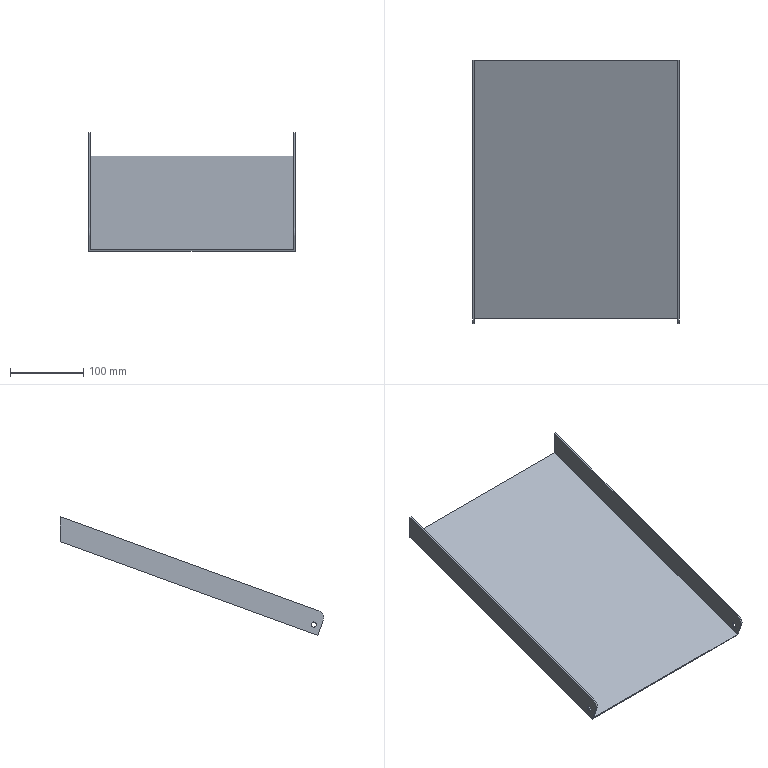Part | NX | features HB 2 | 1 solid | 14 faces | box 281 x 359.033 x 161.773 mm | volume 255383 mm3 | plane 10 | cylinder 4 | commonest cylinder face diameters 7 x2 20 x2
STEP:
#1=CARTESIAN_POINT('',(285.,-685.612,-380.836));
#2=VERTEX_POINT('',#1);
#3=CARTESIAN_POINT('',(285.,-685.612,-377.336));
#4=DIRECTION('',(-1.,0.,0.));
#5=DIRECTION('',(0.,0.,-1.));
#6=AXIS2_PLACEMENT_3D('',#3,#4,#5);
#7=CIRCLE('',#6,3.5);
#8=EDGE_CURVE('',#2,#2,#7,.T.);
#9=ORIENTED_EDGE('',*,*,#8,.T.);
#10=EDGE_LOOP('',(#9));
#11=FACE_BOUND('',#10,.T.);
#12=CARTESIAN_POINT('',(285.,-691.589,-390.154));
#13=VERTEX_POINT('',#12);
#14=CARTESIAN_POINT('',(285.,-340.,-262.186));
#15=VERTEX_POINT('',#14);
#16=CARTESIAN_POINT('',(285.,-379.611,-276.603));
#17=DIRECTION('',(0.,0.9397,0.342));
#18=VECTOR('',#17,1000.);
#19=LINE('',#16,#18);
#20=EDGE_CURVE('',#13,#15,#19,.T.);
#21=ORIENTED_EDGE('',*,*,#20,.T.);
#22=CARTESIAN_POINT('',(285.,-340.,-230.26));
#23=VERTEX_POINT('',#22);
#24=CARTESIAN_POINT('',(285.,-340.,-276.603));
#25=DIRECTION('',(0.,0.,1.));
#26=VECTOR('',#25,1000.);
#27=LINE('',#24,#26);
#28=EDGE_CURVE('',#15,#23,#27,.T.);
#29=ORIENTED_EDGE('',*,*,#28,.T.);
#30=CARTESIAN_POINT('',(285.,-692.453,-358.543));
#31=VERTEX_POINT('',#30);
#32=CARTESIAN_POINT('',(285.,-389.872,-248.412));
#33=DIRECTION('',(0.,-0.9397,-0.342));
#34=VECTOR('',#33,1000.);
#35=LINE('',#32,#34);
#36=EDGE_CURVE('',#23,#31,#35,.T.);
#37=ORIENTED_EDGE('',*,*,#36,.T.);
#38=CARTESIAN_POINT('',(285.,-698.43,-371.36));
#39=VERTEX_POINT('',#38);
#40=CARTESIAN_POINT('',(285.,-689.033,-367.939));
#41=DIRECTION('',(1.,0.,0.));
#42=DIRECTION('',(0.,0.,-1.));
#43=AXIS2_PLACEMENT_3D('',#40,#41,#42);
#44=CIRCLE('',#43,10.);
#45=EDGE_CURVE('',#31,#39,#44,.T.);
#46=ORIENTED_EDGE('',*,*,#45,.T.);
#47=CARTESIAN_POINT('',(285.,-691.589,-390.154));
#48=DIRECTION('',(0.,0.342,-0.9397));
#49=VECTOR('',#48,1000.);
#50=LINE('',#47,#49);
#51=EDGE_CURVE('',#39,#13,#50,.T.);
#52=ORIENTED_EDGE('',*,*,#51,.T.);
#53=EDGE_LOOP('',(#21,#29,#37,#46,#52));
#54=FACE_BOUND('',#53,.T.);
#55=CARTESIAN_POINT('',(285.,-379.611,-276.603));
#56=DIRECTION('',(1.,0.,0.));
#57=DIRECTION('',(0.,0.08716,0.9962));
#58=AXIS2_PLACEMENT_3D('',#55,#56,#57);
#59=PLANE('',#58);
#60=ADVANCED_FACE('',(#11,#54),#59,.T.);
#61=CARTESIAN_POINT('',(562.,-340.,-230.26));
#62=VERTEX_POINT('',#61);
#63=CARTESIAN_POINT('',(564.,-340.,-230.26));
#64=VERTEX_POINT('',#63);
#65=CARTESIAN_POINT('',(562.,-340.,-230.26));
#66=DIRECTION('',(1.,0.,0.));
#67=VECTOR('',#66,1000.);
#68=LINE('',#65,#67);
#69=EDGE_CURVE('',#62,#64,#68,.T.);
#70=ORIENTED_EDGE('',*,*,#69,.F.);
#71=CARTESIAN_POINT('',(562.,-692.453,-358.543));
#72=VERTEX_POINT('',#71);
#73=CARTESIAN_POINT('',(562.,-389.872,-248.412));
#74=DIRECTION('',(0.,-0.9397,-0.342));
#75=VECTOR('',#74,1000.);
#76=LINE('',#73,#75);
#77=EDGE_CURVE('',#62,#72,#76,.T.);
#78=ORIENTED_EDGE('',*,*,#77,.T.);
#79=CARTESIAN_POINT('',(564.,-692.453,-358.543));
#80=VERTEX_POINT('',#79);
#81=CARTESIAN_POINT('',(562.,-692.453,-358.543));
#82=DIRECTION('',(1.,0.,0.));
#83=VECTOR('',#82,1000.);
#84=LINE('',#81,#83);
#85=EDGE_CURVE('',#72,#80,#84,.T.);
#86=ORIENTED_EDGE('',*,*,#85,.T.);
#87=CARTESIAN_POINT('',(564.,-389.872,-248.412));
#88=DIRECTION('',(0.,-0.9397,-0.342));
#89=VECTOR('',#88,1000.);
#90=LINE('',#87,#89);
#91=EDGE_CURVE('',#64,#80,#90,.T.);
#92=ORIENTED_EDGE('',*,*,#91,.F.);
#93=EDGE_LOOP('',(#70,#78,#86,#92));
#94=FACE_BOUND('',#93,.T.);
#95=CARTESIAN_POINT('',(562.,-389.872,-248.412));
#96=DIRECTION('',(0.,0.342,-0.9397));
#97=DIRECTION('',(0.,-0.9397,-0.342));
#98=AXIS2_PLACEMENT_3D('',#95,#96,#97);
#99=PLANE('',#98);
#100=ADVANCED_FACE('',(#94),#99,.F.);
#101=CARTESIAN_POINT('',(562.,-685.307,-373.85));
#102=VERTEX_POINT('',#101);
#103=CARTESIAN_POINT('',(562.,-685.612,-377.336));
#104=DIRECTION('',(1.,0.,0.));
#105=DIRECTION('',(0.,0.08716,0.9962));
#106=AXIS2_PLACEMENT_3D('',#103,#104,#105);
#107=CIRCLE('',#106,3.5);
#108=EDGE_CURVE('',#102,#102,#107,.T.);
#109=ORIENTED_EDGE('',*,*,#108,.T.);
#110=EDGE_LOOP('',(#109));
#111=FACE_BOUND('',#110,.T.);
#112=ORIENTED_EDGE('',*,*,#77,.F.);
#113=CARTESIAN_POINT('',(562.,-340.,-262.186));
#114=VERTEX_POINT('',#113);
#115=CARTESIAN_POINT('',(562.,-340.,-276.603));
#116=DIRECTION('',(0.,0.,-1.));
#117=VECTOR('',#116,1000.);
#118=LINE('',#115,#117);
#119=EDGE_CURVE('',#62,#114,#118,.T.);
#120=ORIENTED_EDGE('',*,*,#119,.T.);
#121=CARTESIAN_POINT('',(562.,-691.589,-390.154));
#122=VERTEX_POINT('',#121);
#123=CARTESIAN_POINT('',(562.,-379.611,-276.603));
#124=DIRECTION('',(0.,-0.9397,-0.342));
#125=VECTOR('',#124,1000.);
#126=LINE('',#123,#125);
#127=EDGE_CURVE('',#114,#122,#126,.T.);
#128=ORIENTED_EDGE('',*,*,#127,.T.);
#129=CARTESIAN_POINT('',(562.,-698.43,-371.36));
#130=VERTEX_POINT('',#129);
#131=CARTESIAN_POINT('',(562.,-691.589,-390.154));
#132=DIRECTION('',(0.,0.342,-0.9397));
#133=VECTOR('',#132,1000.);
#134=LINE('',#131,#133);
#135=EDGE_CURVE('',#130,#122,#134,.T.);
#136=ORIENTED_EDGE('',*,*,#135,.F.);
#137=CARTESIAN_POINT('',(562.,-689.033,-367.939));
#138=DIRECTION('',(-1.,0.,0.));
#139=DIRECTION('',(0.,0.08716,0.9962));
#140=AXIS2_PLACEMENT_3D('',#137,#138,#139);
#141=CIRCLE('',#140,10.);
#142=EDGE_CURVE('',#130,#72,#141,.T.);
#143=ORIENTED_EDGE('',*,*,#142,.T.);
#144=EDGE_LOOP('',(#112,#120,#128,#136,#143));
#145=FACE_BOUND('',#144,.T.);
#146=CARTESIAN_POINT('',(562.,-379.611,-276.603));
#147=DIRECTION('',(-1.,0.,0.));
#148=DIRECTION('',(0.,0.08716,0.9962));
#149=AXIS2_PLACEMENT_3D('',#146,#147,#148);
#150=PLANE('',#149);
#151=ADVANCED_FACE('',(#111,#145),#150,.T.);
#152=CARTESIAN_POINT('',(564.,-685.307,-373.85));
#153=VERTEX_POINT('',#152);
#154=CARTESIAN_POINT('',(564.,-685.612,-377.336));
#155=DIRECTION('',(1.,0.,0.));
#156=DIRECTION('',(0.,0.08716,0.9962));
#157=AXIS2_PLACEMENT_3D('',#154,#155,#156);
#158=CIRCLE('',#157,3.5);
#159=EDGE_CURVE('',#153,#153,#158,.T.);
#160=ORIENTED_EDGE('',*,*,#159,.F.);
#161=EDGE_LOOP('',(#160));
#162=FACE_BOUND('',#161,.T.);
#163=CARTESIAN_POINT('',(564.,-340.,-264.314));
#164=VERTEX_POINT('',#163);
#165=CARTESIAN_POINT('',(564.,-340.,-276.603));
#166=DIRECTION('',(0.,0.,-1.));
#167=VECTOR('',#166,1000.);
#168=LINE('',#165,#167);
#169=EDGE_CURVE('',#64,#164,#168,.T.);
#170=ORIENTED_EDGE('',*,*,#169,.F.);
#171=ORIENTED_EDGE('',*,*,#91,.T.);
#172=CARTESIAN_POINT('',(564.,-698.43,-371.36));
#173=VERTEX_POINT('',#172);
#174=CARTESIAN_POINT('',(564.,-689.033,-367.939));
#175=DIRECTION('',(1.,0.,0.));
#176=DIRECTION('',(0.,0.08716,0.9962));
#177=AXIS2_PLACEMENT_3D('',#174,#175,#176);
#178=CIRCLE('',#177,10.);
#179=EDGE_CURVE('',#80,#173,#178,.T.);
#180=ORIENTED_EDGE('',*,*,#179,.T.);
#181=CARTESIAN_POINT('',(564.,-690.905,-392.033));
#182=VERTEX_POINT('',#181);
#183=CARTESIAN_POINT('',(564.,-691.589,-390.154));
#184=DIRECTION('',(0.,0.342,-0.9397));
#185=VECTOR('',#184,1000.);
#186=LINE('',#183,#185);
#187=EDGE_CURVE('',#173,#182,#186,.T.);
#188=ORIENTED_EDGE('',*,*,#187,.T.);
#189=CARTESIAN_POINT('',(564.,-378.927,-278.482));
#190=DIRECTION('',(0.,0.9397,0.342));
#191=VECTOR('',#190,1000.);
#192=LINE('',#189,#191);
#193=EDGE_CURVE('',#182,#164,#192,.T.);
#194=ORIENTED_EDGE('',*,*,#193,.T.);
#195=EDGE_LOOP('',(#170,#171,#180,#188,#194));
#196=FACE_BOUND('',#195,.T.);
#197=CARTESIAN_POINT('',(564.,-379.611,-276.603));
#198=DIRECTION('',(-1.,0.,0.));
#199=DIRECTION('',(0.,-0.08716,-0.9962));
#200=AXIS2_PLACEMENT_3D('',#197,#198,#199);
#201=PLANE('',#200);
#202=ADVANCED_FACE('',(#162,#196),#201,.F.);
#203=CARTESIAN_POINT('',(283.,-340.,-264.314));
#204=VERTEX_POINT('',#203);
#205=CARTESIAN_POINT('',(283.,-690.905,-392.033));
#206=VERTEX_POINT('',#205);
#207=CARTESIAN_POINT('',(283.,-378.927,-278.482));
#208=DIRECTION('',(0.,-0.9397,-0.342));
#209=VECTOR('',#208,1000.);
#210=LINE('',#207,#209);
#211=EDGE_CURVE('',#204,#206,#210,.T.);
#212=ORIENTED_EDGE('',*,*,#211,.F.);
#213=CARTESIAN_POINT('',(522.,-340.,-264.314));
#214=DIRECTION('',(-1.,0.,0.));
#215=VECTOR('',#214,1000.);
#216=LINE('',#213,#215);
#217=EDGE_CURVE('',#164,#204,#216,.T.);
#218=ORIENTED_EDGE('',*,*,#217,.F.);
#219=ORIENTED_EDGE('',*,*,#193,.F.);
#220=CARTESIAN_POINT('',(522.,-690.905,-392.033));
#221=DIRECTION('',(1.,0.,0.));
#222=VECTOR('',#221,1000.);
#223=LINE('',#220,#222);
#224=EDGE_CURVE('',#206,#182,#223,.T.);
#225=ORIENTED_EDGE('',*,*,#224,.F.);
#226=EDGE_LOOP('',(#212,#218,#219,#225));
#227=FACE_BOUND('',#226,.T.);
#228=CARTESIAN_POINT('',(522.,-378.927,-278.482));
#229=DIRECTION('',(0.,-0.342,0.9397));
#230=DIRECTION('',(-1.,0.,0.));
#231=AXIS2_PLACEMENT_3D('',#228,#229,#230);
#232=PLANE('',#231);
#233=ADVANCED_FACE('',(#227),#232,.F.);
#234=CARTESIAN_POINT('',(522.,-340.,-262.186));
#235=DIRECTION('',(-1.,0.,0.));
#236=VECTOR('',#235,1000.);
#237=LINE('',#234,#236);
#238=EDGE_CURVE('',#114,#15,#237,.T.);
#239=ORIENTED_EDGE('',*,*,#238,.T.);
#240=ORIENTED_EDGE('',*,*,#20,.F.);
#241=CARTESIAN_POINT('',(522.,-691.589,-390.154));
#242=DIRECTION('',(1.,0.,0.));
#243=VECTOR('',#242,1000.);
#244=LINE('',#241,#243);
#245=EDGE_CURVE('',#13,#122,#244,.T.);
#246=ORIENTED_EDGE('',*,*,#245,.T.);
#247=ORIENTED_EDGE('',*,*,#127,.F.);
#248=EDGE_LOOP('',(#239,#240,#246,#247));
#249=FACE_BOUND('',#248,.T.);
#250=CARTESIAN_POINT('',(522.,-379.611,-276.603));
#251=DIRECTION('',(0.,-0.342,0.9397));
#252=DIRECTION('',(-1.,0.,0.));
#253=AXIS2_PLACEMENT_3D('',#250,#251,#252);
#254=PLANE('',#253);
#255=ADVANCED_FACE('',(#249),#254,.T.);
#256=CARTESIAN_POINT('',(283.,-340.,-230.26));
#257=VERTEX_POINT('',#256);
#258=CARTESIAN_POINT('',(275.,-340.,-230.26));
#259=DIRECTION('',(1.,0.,0.));
#260=VECTOR('',#259,1000.);
#261=LINE('',#258,#260);
#262=EDGE_CURVE('',#257,#23,#261,.T.);
#263=ORIENTED_EDGE('',*,*,#262,.F.);
#264=CARTESIAN_POINT('',(283.,-692.453,-358.543));
#265=VERTEX_POINT('',#264);
#266=CARTESIAN_POINT('',(283.,-389.872,-248.412));
#267=DIRECTION('',(0.,-0.9397,-0.342));
#268=VECTOR('',#267,1000.);
#269=LINE('',#266,#268);
#270=EDGE_CURVE('',#257,#265,#269,.T.);
#271=ORIENTED_EDGE('',*,*,#270,.T.);
#272=CARTESIAN_POINT('',(330.,-692.453,-358.543));
#273=DIRECTION('',(1.,0.,0.));
#274=VECTOR('',#273,1000.);
#275=LINE('',#272,#274);
#276=EDGE_CURVE('',#265,#31,#275,.T.);
#277=ORIENTED_EDGE('',*,*,#276,.T.);
#278=ORIENTED_EDGE('',*,*,#36,.F.);
#279=EDGE_LOOP('',(#263,#271,#277,#278));
#280=FACE_BOUND('',#279,.T.);
#281=CARTESIAN_POINT('',(275.,-389.872,-248.412));
#282=DIRECTION('',(0.,0.342,-0.9397));
#283=DIRECTION('',(0.,-0.9397,-0.342));
#284=AXIS2_PLACEMENT_3D('',#281,#282,#283);
#285=PLANE('',#284);
#286=ADVANCED_FACE('',(#280),#285,.F.);
#287=CARTESIAN_POINT('',(283.,-685.612,-380.836));
#288=VERTEX_POINT('',#287);
#289=CARTESIAN_POINT('',(283.,-685.612,-377.336));
#290=DIRECTION('',(1.,0.,0.));
#291=DIRECTION('',(0.,0.,-1.));
#292=AXIS2_PLACEMENT_3D('',#289,#290,#291);
#293=CIRCLE('',#292,3.5);
#294=EDGE_CURVE('',#288,#288,#293,.T.);
#295=ORIENTED_EDGE('',*,*,#294,.T.);
#296=EDGE_LOOP('',(#295));
#297=FACE_BOUND('',#296,.T.);
#298=CARTESIAN_POINT('',(283.,-340.,-276.603));
#299=DIRECTION('',(0.,0.,1.));
#300=VECTOR('',#299,1000.);
#301=LINE('',#298,#300);
#302=EDGE_CURVE('',#204,#257,#301,.T.);
#303=ORIENTED_EDGE('',*,*,#302,.F.);
#304=ORIENTED_EDGE('',*,*,#211,.T.);
#305=CARTESIAN_POINT('',(283.,-698.43,-371.36));
#306=VERTEX_POINT('',#305);
#307=CARTESIAN_POINT('',(283.,-691.589,-390.154));
#308=DIRECTION('',(0.,0.342,-0.9397));
#309=VECTOR('',#308,1000.);
#310=LINE('',#307,#309);
#311=EDGE_CURVE('',#306,#206,#310,.T.);
#312=ORIENTED_EDGE('',*,*,#311,.F.);
#313=CARTESIAN_POINT('',(283.,-689.033,-367.939));
#314=DIRECTION('',(-1.,0.,0.));
#315=DIRECTION('',(0.,0.,-1.));
#316=AXIS2_PLACEMENT_3D('',#313,#314,#315);
#317=CIRCLE('',#316,10.);
#318=EDGE_CURVE('',#306,#265,#317,.T.);
#319=ORIENTED_EDGE('',*,*,#318,.T.);
#320=ORIENTED_EDGE('',*,*,#270,.F.);
#321=EDGE_LOOP('',(#303,#304,#312,#319,#320));
#322=FACE_BOUND('',#321,.T.);
#323=CARTESIAN_POINT('',(283.,-379.611,-276.603));
#324=DIRECTION('',(1.,0.,0.));
#325=DIRECTION('',(0.,0.08716,0.9962));
#326=AXIS2_PLACEMENT_3D('',#323,#324,#325);
#327=PLANE('',#326);
#328=ADVANCED_FACE('',(#297,#322),#327,.F.);
#329=ORIENTED_EDGE('',*,*,#108,.F.);
#330=EDGE_LOOP('',(#329));
#331=FACE_BOUND('',#330,.T.);
#332=ORIENTED_EDGE('',*,*,#159,.T.);
#333=EDGE_LOOP('',(#332));
#334=FACE_BOUND('',#333,.T.);
#335=CARTESIAN_POINT('',(1166.,-685.612,-377.336));
#336=DIRECTION('',(-1.,0.,0.));
#337=DIRECTION('',(0.,-0.08716,-0.9962));
#338=AXIS2_PLACEMENT_3D('',#335,#336,#337);
#339=CYLINDRICAL_SURFACE('',#338,3.5);
#340=ADVANCED_FACE('',(#331,#334),#339,.F.);
#341=ORIENTED_EDGE('',*,*,#142,.F.);
#342=CARTESIAN_POINT('',(522.,-698.43,-371.36));
#343=DIRECTION('',(-1.,0.,0.));
#344=VECTOR('',#343,1000.);
#345=LINE('',#342,#344);
#346=EDGE_CURVE('',#173,#130,#345,.T.);
#347=ORIENTED_EDGE('',*,*,#346,.F.);
#348=ORIENTED_EDGE('',*,*,#179,.F.);
#349=ORIENTED_EDGE('',*,*,#85,.F.);
#350=EDGE_LOOP('',(#341,#347,#348,#349));
#351=FACE_BOUND('',#350,.T.);
#352=CARTESIAN_POINT('',(562.,-689.033,-367.939));
#353=DIRECTION('',(1.,0.,0.));
#354=DIRECTION('',(0.,0.08716,0.9962));
#355=AXIS2_PLACEMENT_3D('',#352,#353,#354);
#356=CYLINDRICAL_SURFACE('',#355,10.);
#357=ADVANCED_FACE('',(#351),#356,.T.);
#358=ORIENTED_EDGE('',*,*,#245,.F.);
#359=ORIENTED_EDGE('',*,*,#51,.F.);
#360=CARTESIAN_POINT('',(588.,-698.43,-371.36));
#361=DIRECTION('',(-1.,0.,0.));
#362=VECTOR('',#361,1000.);
#363=LINE('',#360,#362);
#364=EDGE_CURVE('',#39,#306,#363,.T.);
#365=ORIENTED_EDGE('',*,*,#364,.T.);
#366=ORIENTED_EDGE('',*,*,#311,.T.);
#367=ORIENTED_EDGE('',*,*,#224,.T.);
#368=ORIENTED_EDGE('',*,*,#187,.F.);
#369=ORIENTED_EDGE('',*,*,#346,.T.);
#370=ORIENTED_EDGE('',*,*,#135,.T.);
#371=EDGE_LOOP('',(#358,#359,#365,#366,#367,#368,#369,#370));
#372=FACE_BOUND('',#371,.T.);
#373=CARTESIAN_POINT('',(522.,-691.589,-390.154));
#374=DIRECTION('',(0.,0.9397,0.342));
#375=DIRECTION('',(0.,0.342,-0.9397));
#376=AXIS2_PLACEMENT_3D('',#373,#374,#375);
#377=PLANE('',#376);
#378=ADVANCED_FACE('',(#372),#377,.F.);
#379=ORIENTED_EDGE('',*,*,#45,.F.);
#380=ORIENTED_EDGE('',*,*,#276,.F.);
#381=ORIENTED_EDGE('',*,*,#318,.F.);
#382=ORIENTED_EDGE('',*,*,#364,.F.);
#383=EDGE_LOOP('',(#379,#380,#381,#382));
#384=FACE_BOUND('',#383,.T.);
#385=CARTESIAN_POINT('',(588.,-689.033,-367.939));
#386=DIRECTION('',(-1.,0.,0.));
#387=DIRECTION('',(0.,-0.08716,-0.9962));
#388=AXIS2_PLACEMENT_3D('',#385,#386,#387);
#389=CYLINDRICAL_SURFACE('',#388,10.);
#390=ADVANCED_FACE('',(#384),#389,.T.);
#391=ORIENTED_EDGE('',*,*,#8,.F.);
#392=EDGE_LOOP('',(#391));
#393=FACE_BOUND('',#392,.T.);
#394=ORIENTED_EDGE('',*,*,#294,.F.);
#395=EDGE_LOOP('',(#394));
#396=FACE_BOUND('',#395,.T.);
#397=CARTESIAN_POINT('',(1180.,-685.612,-377.336));
#398=DIRECTION('',(-1.,0.,0.));
#399=DIRECTION('',(0.,-0.08716,-0.9962));
#400=AXIS2_PLACEMENT_3D('',#397,#398,#399);
#401=CYLINDRICAL_SURFACE('',#400,3.5);
#402=ADVANCED_FACE('',(#393,#396),#401,.F.);
#403=ORIENTED_EDGE('',*,*,#69,.T.);
#404=ORIENTED_EDGE('',*,*,#169,.T.);
#405=ORIENTED_EDGE('',*,*,#217,.T.);
#406=ORIENTED_EDGE('',*,*,#302,.T.);
#407=ORIENTED_EDGE('',*,*,#262,.T.);
#408=ORIENTED_EDGE('',*,*,#28,.F.);
#409=ORIENTED_EDGE('',*,*,#238,.F.);
#410=ORIENTED_EDGE('',*,*,#119,.F.);
#411=EDGE_LOOP('',(#403,#404,#405,#406,#407,#408,#409,#410));
#412=FACE_BOUND('',#411,.T.);
#413=CARTESIAN_POINT('',(130.,-340.,60.));
#414=DIRECTION('',(0.,1.,0.));
#415=DIRECTION('',(0.,0.,-1.));
#416=AXIS2_PLACEMENT_3D('',#413,#414,#415);
#417=PLANE('',#416);
#418=ADVANCED_FACE('',(#412),#417,.T.);
#419=CLOSED_SHELL('',(#60,#100,#151,#202,#233,#255,#286,#328,#340,#357,#378,#390,#402,#418));
#420=MANIFOLD_SOLID_BREP('',#419);
#421=(LENGTH_UNIT()NAMED_UNIT(*)SI_UNIT(.MILLI.,.METRE.));
#422=UNCERTAINTY_MEASURE_WITH_UNIT(LENGTH_MEASURE(0.00001),#421,'','');
#423=(NAMED_UNIT(*)PLANE_ANGLE_UNIT()SI_UNIT($,.RADIAN.));
#424=(NAMED_UNIT(*)SI_UNIT($,.STERADIAN.)SOLID_ANGLE_UNIT());
#425=(GEOMETRIC_REPRESENTATION_CONTEXT(3)GLOBAL_UNCERTAINTY_ASSIGNED_CONTEXT((#422))GLOBAL_UNIT_ASSIGNED_CONTEXT((#421,#423,#424))REPRESENTATION_CONTEXT('',''));
#426=ADVANCED_BREP_SHAPE_REPRESENTATION('',(#420),#425);